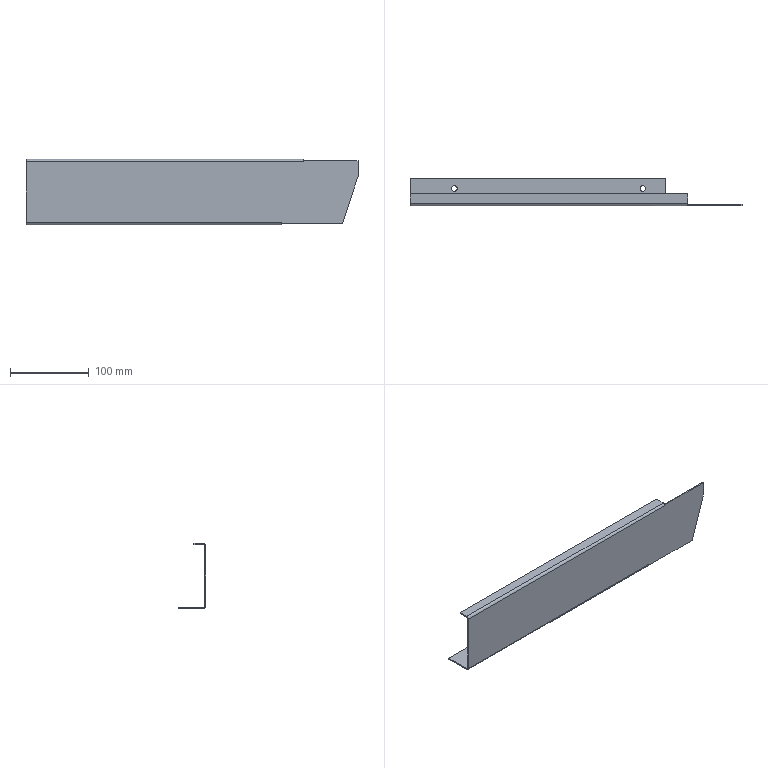Part | STEP file | Top flange baffle (inner bend) | 1 solid | 31 faces | box 422.833 x 35 x 83 mm | volume 73791 mm3 | plane 23 | cylinder 8 | commonest cylinder face diameters 7 x4 3 x2 6 x2